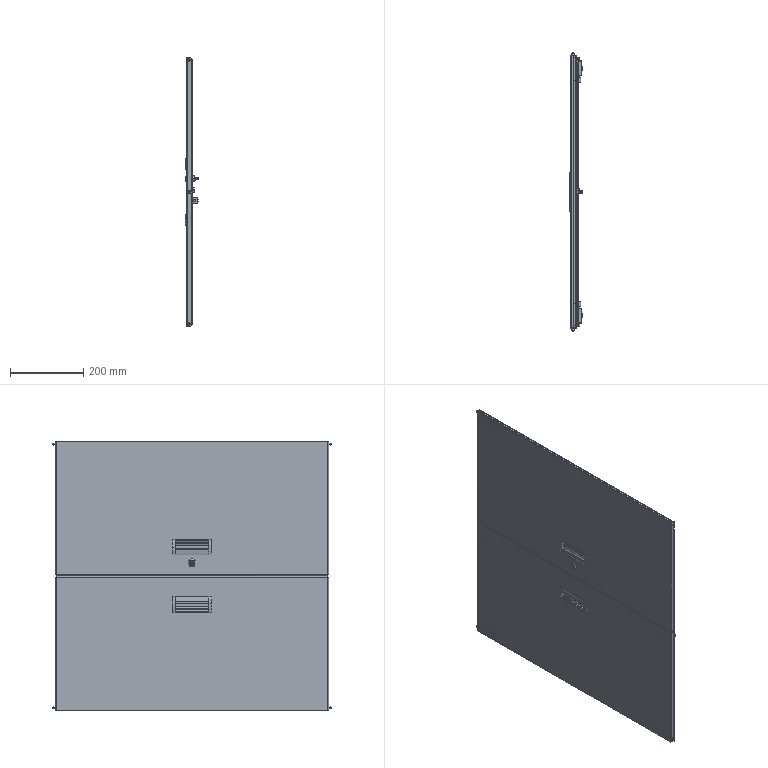Part | SolidWorks | 25 solids | 704 faces | box 37.5 x 764 x 737 mm | volume 1042688 mm3 | plane 394 | cylinder 280 | cone 14 | torus 8 | spline 8 | commonest cylinder face diameters 1 x36 7 x23 0.6 x21 2.5 x16 3.2 x16 5.5 x16